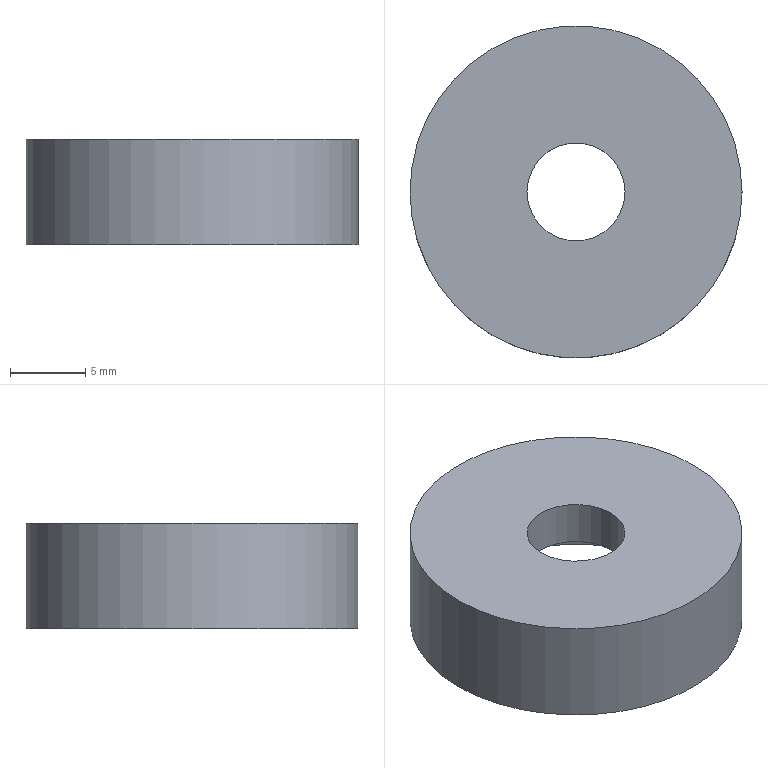Part | NX | features EXTRUDE 2, DATUM_CSYS 1, LINKED_FACE 1, SKETCH 1, UNITE 1 | 1 solid | 6 faces | box 22 x 22 x 7 mm | volume 1632 mm3 | cylinder 3 | plane 3 | commonest cylinder face diameters 6.5 x1 17.2 x1 22 x1
STEP:
#1=CARTESIAN_POINT('',(11.,0.,0.));
#2=VERTEX_POINT('',#1);
#3=CARTESIAN_POINT('',(0.,0.,0.));
#4=DIRECTION('',(0.,0.,-1.));
#5=DIRECTION('',(1.,0.,0.));
#6=AXIS2_PLACEMENT_3D('',#3,#4,#5);
#7=CIRCLE('',#6,11.);
#8=EDGE_CURVE('',#2,#2,#7,.T.);
#9=ORIENTED_EDGE('',*,*,#8,.F.);
#10=EDGE_LOOP('',(#9));
#11=FACE_BOUND('',#10,.T.);
#12=CARTESIAN_POINT('',(11.,0.,7.));
#13=VERTEX_POINT('',#12);
#14=CARTESIAN_POINT('',(0.,0.,7.));
#15=DIRECTION('',(0.,0.,-1.));
#16=DIRECTION('',(1.,0.,0.));
#17=AXIS2_PLACEMENT_3D('',#14,#15,#16);
#18=CIRCLE('',#17,11.);
#19=EDGE_CURVE('',#13,#13,#18,.T.);
#20=ORIENTED_EDGE('',*,*,#19,.T.);
#21=EDGE_LOOP('',(#20));
#22=FACE_BOUND('',#21,.T.);
#23=CARTESIAN_POINT('',(0.,0.,0.));
#24=DIRECTION('',(0.,0.,1.));
#25=DIRECTION('',(1.,0.,0.));
#26=AXIS2_PLACEMENT_3D('',#23,#24,#25);
#27=CYLINDRICAL_SURFACE('',#26,11.);
#28=ADVANCED_FACE('',(#11,#22),#27,.T.);
#29=CARTESIAN_POINT('',(-8.6,0.,4.));
#30=VERTEX_POINT('',#29);
#31=CARTESIAN_POINT('',(0.,0.,4.));
#32=DIRECTION('',(0.,0.,1.));
#33=DIRECTION('',(-1.,0.,0.));
#34=AXIS2_PLACEMENT_3D('',#31,#32,#33);
#35=CIRCLE('',#34,8.6);
#36=EDGE_CURVE('',#30,#30,#35,.T.);
#37=ORIENTED_EDGE('',*,*,#36,.T.);
#38=EDGE_LOOP('',(#37));
#39=FACE_BOUND('',#38,.T.);
#40=CARTESIAN_POINT('',(8.6,0.,0.));
#41=VERTEX_POINT('',#40);
#42=CARTESIAN_POINT('',(0.,0.,0.));
#43=DIRECTION('',(0.,0.,1.));
#44=DIRECTION('',(1.,0.,0.));
#45=AXIS2_PLACEMENT_3D('',#42,#43,#44);
#46=CIRCLE('',#45,8.6);
#47=EDGE_CURVE('',#41,#41,#46,.T.);
#48=ORIENTED_EDGE('',*,*,#47,.F.);
#49=EDGE_LOOP('',(#48));
#50=FACE_BOUND('',#49,.T.);
#51=CARTESIAN_POINT('',(0.,0.,0.));
#52=DIRECTION('',(0.,0.,1.));
#53=DIRECTION('',(1.,0.,0.));
#54=AXIS2_PLACEMENT_3D('',#51,#52,#53);
#55=CYLINDRICAL_SURFACE('',#54,8.6);
#56=ADVANCED_FACE('',(#39,#50),#55,.F.);
#57=ORIENTED_EDGE('',*,*,#8,.T.);
#58=EDGE_LOOP('',(#57));
#59=FACE_BOUND('',#58,.T.);
#60=ORIENTED_EDGE('',*,*,#47,.T.);
#61=EDGE_LOOP('',(#60));
#62=FACE_BOUND('',#61,.T.);
#63=CARTESIAN_POINT('',(0.,0.,0.));
#64=DIRECTION('',(0.,0.,-1.));
#65=DIRECTION('',(-1.,0.,0.));
#66=AXIS2_PLACEMENT_3D('',#63,#64,#65);
#67=PLANE('',#66);
#68=ADVANCED_FACE('',(#59,#62),#67,.T.);
#69=CARTESIAN_POINT('',(-3.25,0.,4.));
#70=VERTEX_POINT('',#69);
#71=CARTESIAN_POINT('',(0.,0.,4.));
#72=DIRECTION('',(0.,0.,1.));
#73=DIRECTION('',(-1.,0.,0.));
#74=AXIS2_PLACEMENT_3D('',#71,#72,#73);
#75=CIRCLE('',#74,3.25);
#76=EDGE_CURVE('',#70,#70,#75,.T.);
#77=ORIENTED_EDGE('',*,*,#76,.T.);
#78=EDGE_LOOP('',(#77));
#79=FACE_BOUND('',#78,.T.);
#80=ORIENTED_EDGE('',*,*,#36,.F.);
#81=EDGE_LOOP('',(#80));
#82=FACE_BOUND('',#81,.T.);
#83=CARTESIAN_POINT('',(0.,0.,4.));
#84=DIRECTION('',(0.,0.,-1.));
#85=DIRECTION('',(-1.,0.,0.));
#86=AXIS2_PLACEMENT_3D('',#83,#84,#85);
#87=PLANE('',#86);
#88=ADVANCED_FACE('',(#79,#82),#87,.T.);
#89=ORIENTED_EDGE('',*,*,#76,.F.);
#90=EDGE_LOOP('',(#89));
#91=FACE_BOUND('',#90,.T.);
#92=CARTESIAN_POINT('',(3.25,0.,7.));
#93=VERTEX_POINT('',#92);
#94=CARTESIAN_POINT('',(0.,0.,7.));
#95=DIRECTION('',(0.,0.,1.));
#96=DIRECTION('',(1.,0.,0.));
#97=AXIS2_PLACEMENT_3D('',#94,#95,#96);
#98=CIRCLE('',#97,3.25);
#99=EDGE_CURVE('',#93,#93,#98,.T.);
#100=ORIENTED_EDGE('',*,*,#99,.T.);
#101=EDGE_LOOP('',(#100));
#102=FACE_BOUND('',#101,.T.);
#103=CARTESIAN_POINT('',(0.,0.,7.));
#104=DIRECTION('',(0.,0.,-1.));
#105=DIRECTION('',(-1.,0.,0.));
#106=AXIS2_PLACEMENT_3D('',#103,#104,#105);
#107=CYLINDRICAL_SURFACE('',#106,3.25);
#108=ADVANCED_FACE('',(#91,#102),#107,.F.);
#109=ORIENTED_EDGE('',*,*,#19,.F.);
#110=EDGE_LOOP('',(#109));
#111=FACE_BOUND('',#110,.T.);
#112=ORIENTED_EDGE('',*,*,#99,.F.);
#113=EDGE_LOOP('',(#112));
#114=FACE_BOUND('',#113,.T.);
#115=CARTESIAN_POINT('',(0.,0.,7.));
#116=DIRECTION('',(0.,0.,-1.));
#117=DIRECTION('',(-1.,0.,0.));
#118=AXIS2_PLACEMENT_3D('',#115,#116,#117);
#119=PLANE('',#118);
#120=ADVANCED_FACE('',(#111,#114),#119,.F.);
#121=CLOSED_SHELL('',(#28,#56,#68,#88,#108,#120));
#122=MANIFOLD_SOLID_BREP('',#121);
#123=(LENGTH_UNIT()NAMED_UNIT(*)SI_UNIT(.MILLI.,.METRE.));
#124=UNCERTAINTY_MEASURE_WITH_UNIT(LENGTH_MEASURE(0.00001),#123,'','');
#125=(NAMED_UNIT(*)PLANE_ANGLE_UNIT()SI_UNIT($,.RADIAN.));
#126=(NAMED_UNIT(*)SI_UNIT($,.STERADIAN.)SOLID_ANGLE_UNIT());
#127=(GEOMETRIC_REPRESENTATION_CONTEXT(3)GLOBAL_UNCERTAINTY_ASSIGNED_CONTEXT((#124))GLOBAL_UNIT_ASSIGNED_CONTEXT((#123,#125,#126))REPRESENTATION_CONTEXT('',''));
#128=ADVANCED_BREP_SHAPE_REPRESENTATION('',(#122),#127);